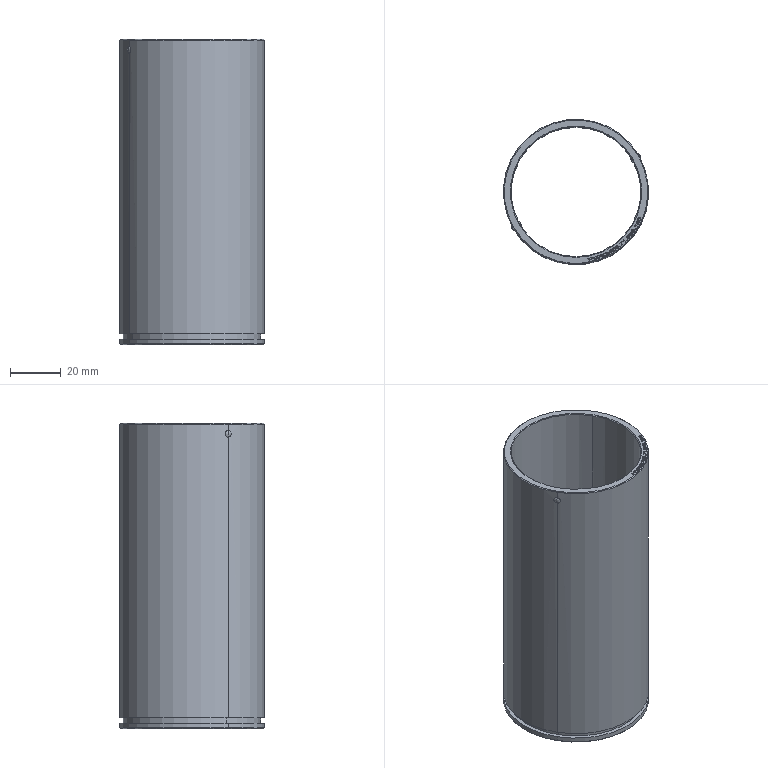Part | NX | features 1 2 | 1 solid | 236 faces | box 57 x 57 x 120 mm | volume 60481 mm3 | plane 110 | spline 102 | cone 8 | cylinder 8 | sphere 8 | commonest cylinder face diameters 57 x4 51 x2 54 x2